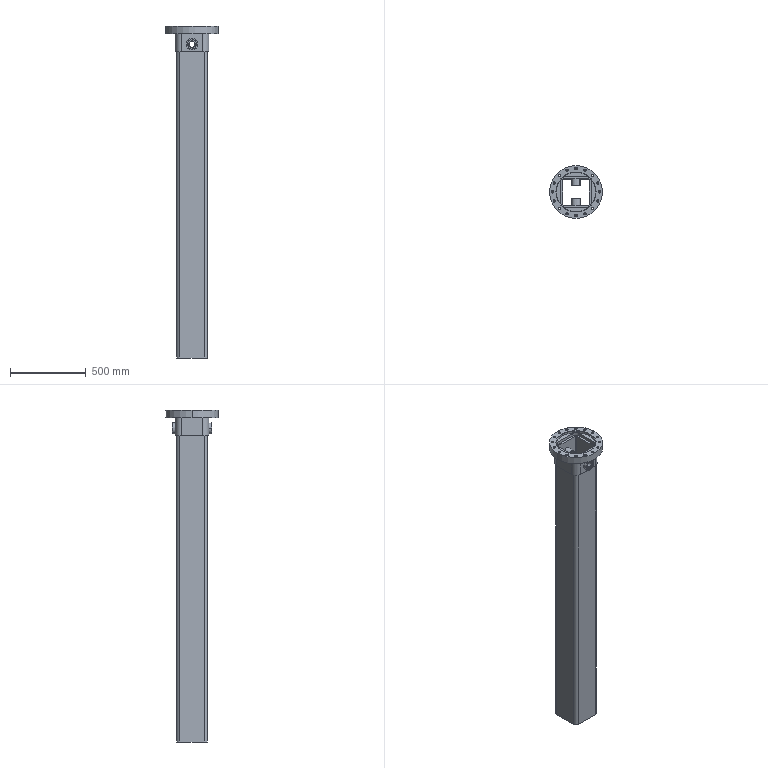Part | SolidWorks | features Cut 4, Chamfer 1, CosmeticWeldCutList 1 | 5 solids | 176 faces | box 348 x 348 x 2185 mm | volume 22246675 mm3 | cylinder 87 | cone 46 | plane 43 | commonest cylinder face diameters 14 x32 60 x24 40 x8 80 x5 16 x4 58 x4